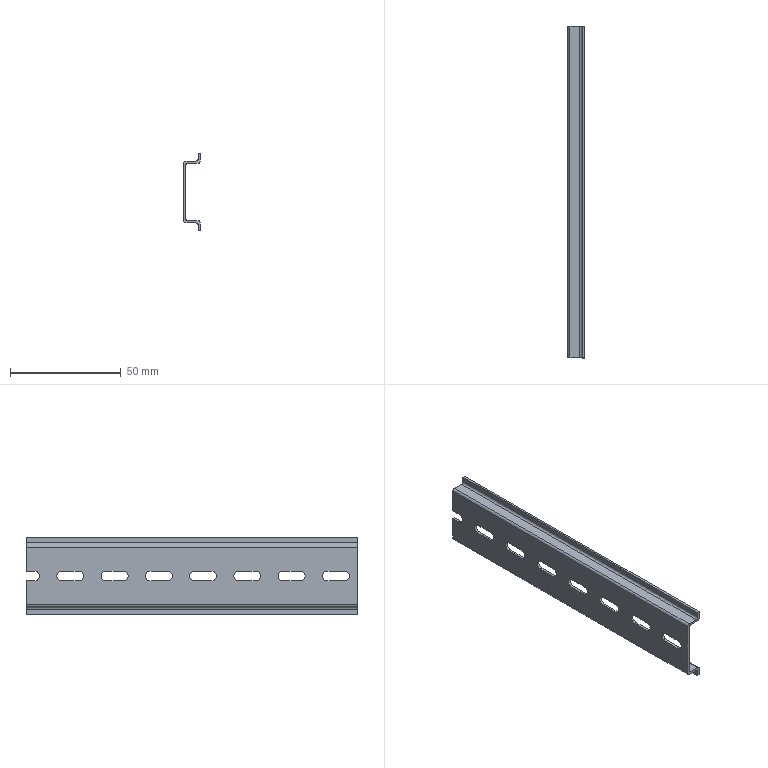Part | STEP file | c45-150 | 1 solid | 54 faces | box 7.5 x 150 x 35 mm | volume 6844 mm3 | plane 31 | cylinder 23 | commonest cylinder face diameters 4.2 x15 2 x8